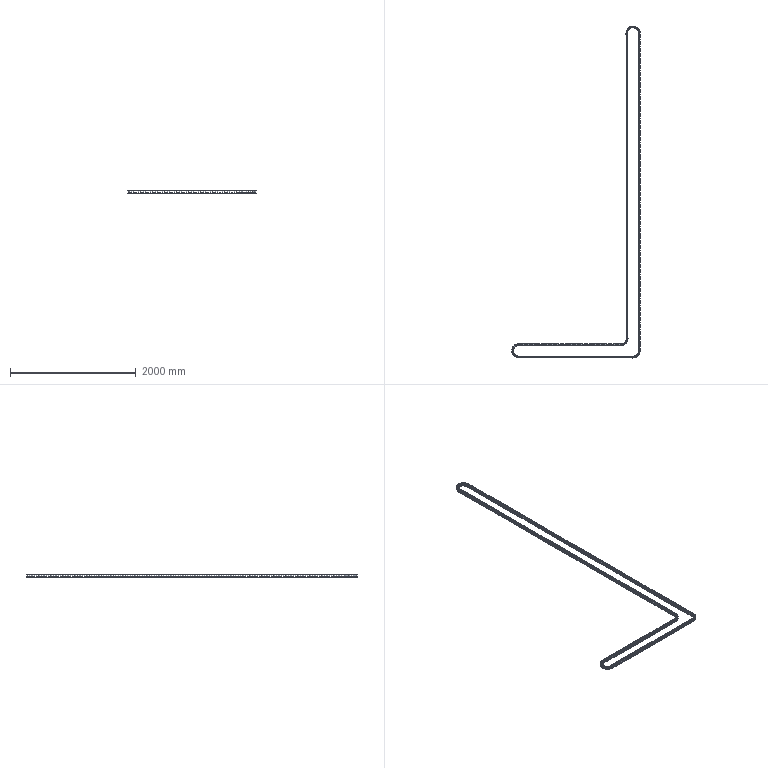Part | STEP file | Inner chain 1-1XG | 187 solids | 5610 faces | volume 4555438 mm3 | cylinder 4114 | plane 1496 | commonest cylinder face diameters 11 x2244 30 x1122 64.25 x748